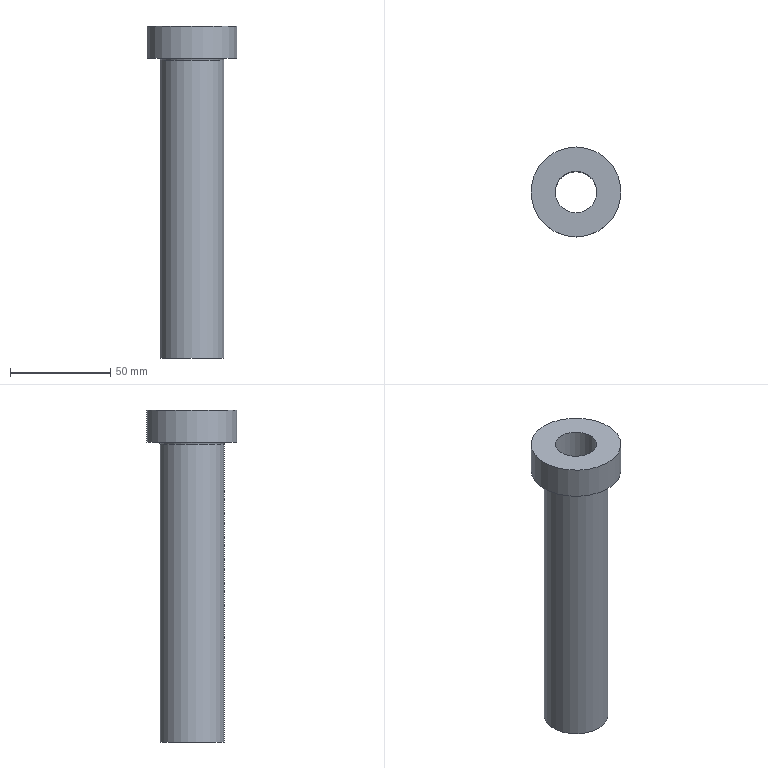Part | NX | features solid 2 | 1 solid | 7 faces | box 45 x 45 x 166 mm | volume 89700 mm3 | plane 3 | cylinder 3 | torus 1 | commonest cylinder face diameters 20.8 x1 32 x1 45 x1
STEP:
#1=CARTESIAN_POINT('',(-425.,276.,-210.));
#2=VERTEX_POINT('',#1);
#3=CARTESIAN_POINT('',(-425.,260.,-210.));
#4=DIRECTION('',(0.,0.,-1.));
#5=DIRECTION('',(0.,1.,0.));
#6=AXIS2_PLACEMENT_3D('',#3,#4,#5);
#7=CIRCLE('',#6,16.);
#8=EDGE_CURVE('',#2,#2,#7,.T.);
#9=ORIENTED_EDGE('',*,*,#8,.T.);
#10=EDGE_LOOP('',(#9));
#11=FACE_BOUND('',#10,.T.);
#12=CARTESIAN_POINT('',(-425.,270.4,-210.));
#13=VERTEX_POINT('',#12);
#14=CARTESIAN_POINT('',(-425.,260.,-210.));
#15=DIRECTION('',(0.,0.,-1.));
#16=DIRECTION('',(0.,1.,0.));
#17=AXIS2_PLACEMENT_3D('',#14,#15,#16);
#18=CIRCLE('',#17,10.4);
#19=EDGE_CURVE('',#13,#13,#18,.T.);
#20=ORIENTED_EDGE('',*,*,#19,.F.);
#21=EDGE_LOOP('',(#20));
#22=FACE_BOUND('',#21,.T.);
#23=CARTESIAN_POINT('',(-425.,270.4,-210.));
#24=DIRECTION('',(0.,0.,-1.));
#25=DIRECTION('',(0.,1.,0.));
#26=AXIS2_PLACEMENT_3D('',#23,#24,#25);
#27=PLANE('',#26);
#28=ADVANCED_FACE('',(#11,#22),#27,.T.);
#29=CARTESIAN_POINT('',(-425.,276.,-61.));
#30=VERTEX_POINT('',#29);
#31=CARTESIAN_POINT('',(-425.,260.,-61.));
#32=DIRECTION('',(0.,0.,-1.));
#33=DIRECTION('',(0.,1.,0.));
#34=AXIS2_PLACEMENT_3D('',#31,#32,#33);
#35=CIRCLE('',#34,16.);
#36=EDGE_CURVE('',#30,#30,#35,.T.);
#37=ORIENTED_EDGE('',*,*,#36,.T.);
#38=EDGE_LOOP('',(#37));
#39=FACE_BOUND('',#38,.T.);
#40=ORIENTED_EDGE('',*,*,#8,.F.);
#41=EDGE_LOOP('',(#40));
#42=FACE_BOUND('',#41,.T.);
#43=CARTESIAN_POINT('',(-425.,260.,-24.));
#44=DIRECTION('',(0.,0.,-1.));
#45=DIRECTION('',(0.,1.,0.));
#46=AXIS2_PLACEMENT_3D('',#43,#44,#45);
#47=CYLINDRICAL_SURFACE('',#46,16.);
#48=ADVANCED_FACE('',(#39,#42),#47,.T.);
#49=CARTESIAN_POINT('',(-425.,277.,-60.));
#50=VERTEX_POINT('',#49);
#51=CARTESIAN_POINT('',(-425.,260.,-60.));
#52=DIRECTION('',(0.,0.,-1.));
#53=DIRECTION('',(0.,1.,0.));
#54=AXIS2_PLACEMENT_3D('',#51,#52,#53);
#55=CIRCLE('',#54,17.);
#56=EDGE_CURVE('',#50,#50,#55,.T.);
#57=ORIENTED_EDGE('',*,*,#56,.T.);
#58=EDGE_LOOP('',(#57));
#59=FACE_BOUND('',#58,.T.);
#60=ORIENTED_EDGE('',*,*,#36,.F.);
#61=EDGE_LOOP('',(#60));
#62=FACE_BOUND('',#61,.T.);
#63=CARTESIAN_POINT('',(-425.,260.,-61.));
#64=DIRECTION('',(0.,0.,-1.));
#65=DIRECTION('',(0.,1.,0.));
#66=AXIS2_PLACEMENT_3D('',#63,#64,#65);
#67=TOROIDAL_SURFACE('',#66,17.,1.);
#68=ADVANCED_FACE('',(#59,#62),#67,.F.);
#69=CARTESIAN_POINT('',(-425.,282.5,-60.));
#70=VERTEX_POINT('',#69);
#71=CARTESIAN_POINT('',(-425.,260.,-60.));
#72=DIRECTION('',(0.,0.,-1.));
#73=DIRECTION('',(0.,1.,0.));
#74=AXIS2_PLACEMENT_3D('',#71,#72,#73);
#75=CIRCLE('',#74,22.5);
#76=EDGE_CURVE('',#70,#70,#75,.T.);
#77=ORIENTED_EDGE('',*,*,#76,.T.);
#78=EDGE_LOOP('',(#77));
#79=FACE_BOUND('',#78,.T.);
#80=ORIENTED_EDGE('',*,*,#56,.F.);
#81=EDGE_LOOP('',(#80));
#82=FACE_BOUND('',#81,.T.);
#83=CARTESIAN_POINT('',(-425.,277.,-60.));
#84=DIRECTION('',(0.,0.,-1.));
#85=DIRECTION('',(0.,1.,0.));
#86=AXIS2_PLACEMENT_3D('',#83,#84,#85);
#87=PLANE('',#86);
#88=ADVANCED_FACE('',(#79,#82),#87,.T.);
#89=CARTESIAN_POINT('',(-425.,282.5,-44.));
#90=VERTEX_POINT('',#89);
#91=CARTESIAN_POINT('',(-425.,260.,-44.));
#92=DIRECTION('',(0.,0.,-1.));
#93=DIRECTION('',(0.,1.,0.));
#94=AXIS2_PLACEMENT_3D('',#91,#92,#93);
#95=CIRCLE('',#94,22.5);
#96=EDGE_CURVE('',#90,#90,#95,.T.);
#97=ORIENTED_EDGE('',*,*,#96,.T.);
#98=EDGE_LOOP('',(#97));
#99=FACE_BOUND('',#98,.T.);
#100=ORIENTED_EDGE('',*,*,#76,.F.);
#101=EDGE_LOOP('',(#100));
#102=FACE_BOUND('',#101,.T.);
#103=CARTESIAN_POINT('',(-425.,260.,-24.));
#104=DIRECTION('',(0.,0.,-1.));
#105=DIRECTION('',(0.,1.,0.));
#106=AXIS2_PLACEMENT_3D('',#103,#104,#105);
#107=CYLINDRICAL_SURFACE('',#106,22.5);
#108=ADVANCED_FACE('',(#99,#102),#107,.T.);
#109=CARTESIAN_POINT('',(-425.,270.4,-44.));
#110=VERTEX_POINT('',#109);
#111=CARTESIAN_POINT('',(-425.,260.,-44.));
#112=DIRECTION('',(0.,0.,-1.));
#113=DIRECTION('',(0.,1.,0.));
#114=AXIS2_PLACEMENT_3D('',#111,#112,#113);
#115=CIRCLE('',#114,10.4);
#116=EDGE_CURVE('',#110,#110,#115,.T.);
#117=ORIENTED_EDGE('',*,*,#116,.T.);
#118=EDGE_LOOP('',(#117));
#119=FACE_BOUND('',#118,.T.);
#120=ORIENTED_EDGE('',*,*,#96,.F.);
#121=EDGE_LOOP('',(#120));
#122=FACE_BOUND('',#121,.T.);
#123=CARTESIAN_POINT('',(-425.,282.5,-44.));
#124=DIRECTION('',(0.,0.,1.));
#125=DIRECTION('',(0.,-1.,0.));
#126=AXIS2_PLACEMENT_3D('',#123,#124,#125);
#127=PLANE('',#126);
#128=ADVANCED_FACE('',(#119,#122),#127,.T.);
#129=ORIENTED_EDGE('',*,*,#19,.T.);
#130=EDGE_LOOP('',(#129));
#131=FACE_BOUND('',#130,.T.);
#132=ORIENTED_EDGE('',*,*,#116,.F.);
#133=EDGE_LOOP('',(#132));
#134=FACE_BOUND('',#133,.T.);
#135=CARTESIAN_POINT('',(-425.,260.,-24.));
#136=DIRECTION('',(0.,0.,-1.));
#137=DIRECTION('',(0.,1.,0.));
#138=AXIS2_PLACEMENT_3D('',#135,#136,#137);
#139=CYLINDRICAL_SURFACE('',#138,10.4);
#140=ADVANCED_FACE('',(#131,#134),#139,.F.);
#141=CLOSED_SHELL('',(#28,#48,#68,#88,#108,#128,#140));
#142=MANIFOLD_SOLID_BREP('',#141);
#143=(LENGTH_UNIT()NAMED_UNIT(*)SI_UNIT(.MILLI.,.METRE.));
#144=UNCERTAINTY_MEASURE_WITH_UNIT(LENGTH_MEASURE(0.00001),#143,'','');
#145=(NAMED_UNIT(*)PLANE_ANGLE_UNIT()SI_UNIT($,.RADIAN.));
#146=(NAMED_UNIT(*)SI_UNIT($,.STERADIAN.)SOLID_ANGLE_UNIT());
#147=(GEOMETRIC_REPRESENTATION_CONTEXT(3)GLOBAL_UNCERTAINTY_ASSIGNED_CONTEXT((#144))GLOBAL_UNIT_ASSIGNED_CONTEXT((#143,#145,#146))REPRESENTATION_CONTEXT('',''));
#148=ADVANCED_BREP_SHAPE_REPRESENTATION('',(#142),#147);